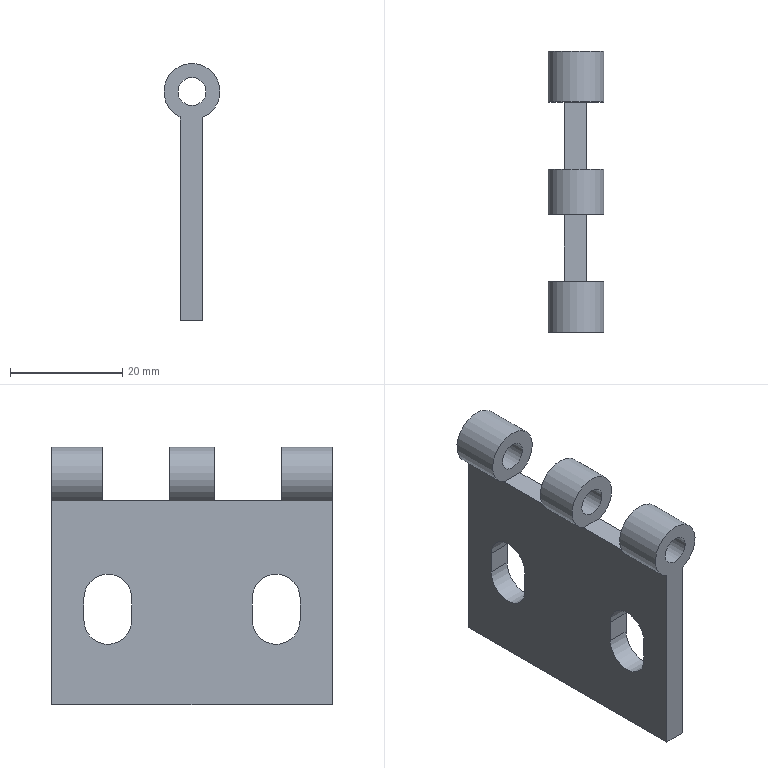Part | NX | features solid 2 | 1 solid | 24 faces | box 10 x 50 x 45.793 mm | volume 8023 mm3 | plane 14 | cylinder 10 | commonest cylinder face diameters 8.5 x4 5 x3 10 x3
STEP:
#1=CARTESIAN_POINT('',(-1603.983,496.,11.257));
#2=VERTEX_POINT('',#1);
#3=CARTESIAN_POINT('',(-1603.983,505.,11.257));
#4=VERTEX_POINT('',#3);
#5=CARTESIAN_POINT('',(-1603.983,485.,11.257));
#6=DIRECTION('',(0.,1.,0.));
#7=VECTOR('',#6,1000.);
#8=LINE('',#5,#7);
#9=EDGE_CURVE('',#2,#4,#8,.T.);
#10=ORIENTED_EDGE('',*,*,#9,.T.);
#11=CARTESIAN_POINT('',(-1604.,505.,11.257));
#12=VERTEX_POINT('',#11);
#13=CARTESIAN_POINT('',(-1604.,505.,11.257));
#14=DIRECTION('',(1.,0.,0.));
#15=VECTOR('',#14,1000.);
#16=LINE('',#13,#15);
#17=EDGE_CURVE('',#12,#4,#16,.T.);
#18=ORIENTED_EDGE('',*,*,#17,.F.);
#19=CARTESIAN_POINT('',(-1604.,455.,11.257));
#20=VERTEX_POINT('',#19);
#21=CARTESIAN_POINT('',(-1604.,505.,11.257));
#22=DIRECTION('',(0.,1.,0.));
#23=VECTOR('',#22,1000.);
#24=LINE('',#21,#23);
#25=EDGE_CURVE('',#12,#20,#24,.F.);
#26=ORIENTED_EDGE('',*,*,#25,.T.);
#27=CARTESIAN_POINT('',(-1603.983,455.,11.257));
#28=VERTEX_POINT('',#27);
#29=CARTESIAN_POINT('',(-1604.,455.,11.257));
#30=DIRECTION('',(1.,0.,0.));
#31=VECTOR('',#30,1000.);
#32=LINE('',#29,#31);
#33=EDGE_CURVE('',#20,#28,#32,.T.);
#34=ORIENTED_EDGE('',*,*,#33,.T.);
#35=CARTESIAN_POINT('',(-1603.983,464.,11.257));
#36=VERTEX_POINT('',#35);
#37=CARTESIAN_POINT('',(-1603.983,445.,11.257));
#38=DIRECTION('',(0.,1.,0.));
#39=VECTOR('',#38,1000.);
#40=LINE('',#37,#39);
#41=EDGE_CURVE('',#28,#36,#40,.T.);
#42=ORIENTED_EDGE('',*,*,#41,.T.);
#43=CARTESIAN_POINT('',(-1600.,464.,11.257));
#44=VERTEX_POINT('',#43);
#45=CARTESIAN_POINT('',(-1604.,464.,11.257));
#46=DIRECTION('',(1.,0.,0.));
#47=VECTOR('',#46,1000.);
#48=LINE('',#45,#47);
#49=EDGE_CURVE('',#36,#44,#48,.T.);
#50=ORIENTED_EDGE('',*,*,#49,.T.);
#51=CARTESIAN_POINT('',(-1600.,476.,11.257));
#52=VERTEX_POINT('',#51);
#53=CARTESIAN_POINT('',(-1600.,505.,11.257));
#54=DIRECTION('',(0.,1.,0.));
#55=VECTOR('',#54,1000.);
#56=LINE('',#53,#55);
#57=EDGE_CURVE('',#52,#44,#56,.F.);
#58=ORIENTED_EDGE('',*,*,#57,.F.);
#59=CARTESIAN_POINT('',(-1603.983,476.,11.257));
#60=VERTEX_POINT('',#59);
#61=CARTESIAN_POINT('',(-1604.,476.,11.257));
#62=DIRECTION('',(1.,0.,0.));
#63=VECTOR('',#62,1000.);
#64=LINE('',#61,#63);
#65=EDGE_CURVE('',#60,#52,#64,.T.);
#66=ORIENTED_EDGE('',*,*,#65,.F.);
#67=CARTESIAN_POINT('',(-1603.983,484.,11.257));
#68=VERTEX_POINT('',#67);
#69=CARTESIAN_POINT('',(-1603.983,465.,11.257));
#70=DIRECTION('',(0.,1.,0.));
#71=VECTOR('',#70,1000.);
#72=LINE('',#69,#71);
#73=EDGE_CURVE('',#60,#68,#72,.T.);
#74=ORIENTED_EDGE('',*,*,#73,.T.);
#75=CARTESIAN_POINT('',(-1600.,484.,11.257));
#76=VERTEX_POINT('',#75);
#77=CARTESIAN_POINT('',(-1604.,484.,11.257));
#78=DIRECTION('',(1.,0.,0.));
#79=VECTOR('',#78,1000.);
#80=LINE('',#77,#79);
#81=EDGE_CURVE('',#68,#76,#80,.T.);
#82=ORIENTED_EDGE('',*,*,#81,.T.);
#83=CARTESIAN_POINT('',(-1600.,496.,11.257));
#84=VERTEX_POINT('',#83);
#85=CARTESIAN_POINT('',(-1600.,505.,11.257));
#86=DIRECTION('',(0.,1.,0.));
#87=VECTOR('',#86,1000.);
#88=LINE('',#85,#87);
#89=EDGE_CURVE('',#84,#76,#88,.F.);
#90=ORIENTED_EDGE('',*,*,#89,.F.);
#91=CARTESIAN_POINT('',(-1604.,496.,11.257));
#92=DIRECTION('',(1.,0.,0.));
#93=VECTOR('',#92,1000.);
#94=LINE('',#91,#93);
#95=EDGE_CURVE('',#2,#84,#94,.T.);
#96=ORIENTED_EDGE('',*,*,#95,.F.);
#97=EDGE_LOOP('',(#10,#18,#26,#34,#42,#50,#58,#66,#74,#82,#90,#96));
#98=FACE_BOUND('',#97,.T.);
#99=CARTESIAN_POINT('',(-1604.,505.,11.257));
#100=DIRECTION('',(0.,0.,-1.));
#101=DIRECTION('',(0.,-1.,0.));
#102=AXIS2_PLACEMENT_3D('',#99,#100,#101);
#103=PLANE('',#102);
#104=ADVANCED_FACE('',(#98),#103,.F.);
#105=CARTESIAN_POINT('',(-1600.,490.75,-10.));
#106=VERTEX_POINT('',#105);
#107=CARTESIAN_POINT('',(-1600.,490.75,-6.));
#108=VERTEX_POINT('',#107);
#109=CARTESIAN_POINT('',(-1600.,490.75,-10.));
#110=DIRECTION('',(0.,0.,1.));
#111=VECTOR('',#110,1000.);
#112=LINE('',#109,#111);
#113=EDGE_CURVE('',#106,#108,#112,.T.);
#114=ORIENTED_EDGE('',*,*,#113,.T.);
#115=CARTESIAN_POINT('',(-1600.,499.25,-6.));
#116=VERTEX_POINT('',#115);
#117=CARTESIAN_POINT('',(-1600.,495.,-6.));
#118=DIRECTION('',(1.,0.,0.));
#119=DIRECTION('',(0.,0.,-1.));
#120=AXIS2_PLACEMENT_3D('',#117,#118,#119);
#121=CIRCLE('',#120,4.25);
#122=EDGE_CURVE('',#116,#108,#121,.T.);
#123=ORIENTED_EDGE('',*,*,#122,.F.);
#124=CARTESIAN_POINT('',(-1600.,499.25,-10.));
#125=VERTEX_POINT('',#124);
#126=CARTESIAN_POINT('',(-1600.,499.25,-10.));
#127=DIRECTION('',(0.,0.,1.));
#128=VECTOR('',#127,1000.);
#129=LINE('',#126,#128);
#130=EDGE_CURVE('',#125,#116,#129,.T.);
#131=ORIENTED_EDGE('',*,*,#130,.F.);
#132=CARTESIAN_POINT('',(-1600.,495.,-10.));
#133=DIRECTION('',(1.,0.,0.));
#134=DIRECTION('',(0.,0.,-1.));
#135=AXIS2_PLACEMENT_3D('',#132,#133,#134);
#136=CIRCLE('',#135,4.25);
#137=EDGE_CURVE('',#106,#125,#136,.T.);
#138=ORIENTED_EDGE('',*,*,#137,.F.);
#139=EDGE_LOOP('',(#114,#123,#131,#138));
#140=FACE_BOUND('',#139,.T.);
#141=CARTESIAN_POINT('',(-1600.,460.75,-10.));
#142=VERTEX_POINT('',#141);
#143=CARTESIAN_POINT('',(-1600.,460.75,-6.));
#144=VERTEX_POINT('',#143);
#145=CARTESIAN_POINT('',(-1600.,460.75,-10.));
#146=DIRECTION('',(0.,0.,1.));
#147=VECTOR('',#146,1000.);
#148=LINE('',#145,#147);
#149=EDGE_CURVE('',#142,#144,#148,.T.);
#150=ORIENTED_EDGE('',*,*,#149,.T.);
#151=CARTESIAN_POINT('',(-1600.,469.25,-6.));
#152=VERTEX_POINT('',#151);
#153=CARTESIAN_POINT('',(-1600.,465.,-6.));
#154=DIRECTION('',(1.,0.,0.));
#155=DIRECTION('',(0.,0.,-1.));
#156=AXIS2_PLACEMENT_3D('',#153,#154,#155);
#157=CIRCLE('',#156,4.25);
#158=EDGE_CURVE('',#152,#144,#157,.T.);
#159=ORIENTED_EDGE('',*,*,#158,.F.);
#160=CARTESIAN_POINT('',(-1600.,469.25,-10.));
#161=VERTEX_POINT('',#160);
#162=CARTESIAN_POINT('',(-1600.,469.25,-10.));
#163=DIRECTION('',(0.,0.,1.));
#164=VECTOR('',#163,1000.);
#165=LINE('',#162,#164);
#166=EDGE_CURVE('',#161,#152,#165,.T.);
#167=ORIENTED_EDGE('',*,*,#166,.F.);
#168=CARTESIAN_POINT('',(-1600.,465.,-10.));
#169=DIRECTION('',(1.,0.,0.));
#170=DIRECTION('',(0.,0.,-1.));
#171=AXIS2_PLACEMENT_3D('',#168,#169,#170);
#172=CIRCLE('',#171,4.25);
#173=EDGE_CURVE('',#142,#161,#172,.T.);
#174=ORIENTED_EDGE('',*,*,#173,.F.);
#175=EDGE_LOOP('',(#150,#159,#167,#174));
#176=FACE_BOUND('',#175,.T.);
#177=CARTESIAN_POINT('',(-1600.,496.,11.159));
#178=VERTEX_POINT('',#177);
#179=CARTESIAN_POINT('',(-1600.,496.,-39.243));
#180=DIRECTION('',(0.,0.,-1.));
#181=VECTOR('',#180,1000.);
#182=LINE('',#179,#181);
#183=EDGE_CURVE('',#178,#84,#182,.F.);
#184=ORIENTED_EDGE('',*,*,#183,.T.);
#185=ORIENTED_EDGE('',*,*,#89,.T.);
#186=CARTESIAN_POINT('',(-1600.,484.,11.159));
#187=VERTEX_POINT('',#186);
#188=CARTESIAN_POINT('',(-1600.,484.,-39.243));
#189=DIRECTION('',(0.,0.,-1.));
#190=VECTOR('',#189,1000.);
#191=LINE('',#188,#190);
#192=EDGE_CURVE('',#187,#76,#191,.F.);
#193=ORIENTED_EDGE('',*,*,#192,.F.);
#194=CARTESIAN_POINT('',(-1600.,476.,11.159));
#195=VERTEX_POINT('',#194);
#196=CARTESIAN_POINT('',(-1600.,465.,11.159));
#197=DIRECTION('',(0.,1.,0.));
#198=VECTOR('',#197,1000.);
#199=LINE('',#196,#198);
#200=EDGE_CURVE('',#195,#187,#199,.T.);
#201=ORIENTED_EDGE('',*,*,#200,.F.);
#202=CARTESIAN_POINT('',(-1600.,476.,-39.243));
#203=DIRECTION('',(0.,0.,-1.));
#204=VECTOR('',#203,1000.);
#205=LINE('',#202,#204);
#206=EDGE_CURVE('',#195,#52,#205,.F.);
#207=ORIENTED_EDGE('',*,*,#206,.T.);
#208=ORIENTED_EDGE('',*,*,#57,.T.);
#209=CARTESIAN_POINT('',(-1600.,464.,11.159));
#210=VERTEX_POINT('',#209);
#211=CARTESIAN_POINT('',(-1600.,464.,-39.243));
#212=DIRECTION('',(0.,0.,-1.));
#213=VECTOR('',#212,1000.);
#214=LINE('',#211,#213);
#215=EDGE_CURVE('',#210,#44,#214,.F.);
#216=ORIENTED_EDGE('',*,*,#215,.F.);
#217=CARTESIAN_POINT('',(-1600.,455.,11.159));
#218=VERTEX_POINT('',#217);
#219=CARTESIAN_POINT('',(-1600.,445.,11.159));
#220=DIRECTION('',(0.,1.,0.));
#221=VECTOR('',#220,1000.);
#222=LINE('',#219,#221);
#223=EDGE_CURVE('',#218,#210,#222,.T.);
#224=ORIENTED_EDGE('',*,*,#223,.F.);
#225=CARTESIAN_POINT('',(-1600.,455.,-25.));
#226=VERTEX_POINT('',#225);
#227=CARTESIAN_POINT('',(-1600.,455.,-39.243));
#228=DIRECTION('',(0.,0.,-1.));
#229=VECTOR('',#228,1000.);
#230=LINE('',#227,#229);
#231=EDGE_CURVE('',#226,#218,#230,.F.);
#232=ORIENTED_EDGE('',*,*,#231,.F.);
#233=CARTESIAN_POINT('',(-1600.,505.,-25.));
#234=VERTEX_POINT('',#233);
#235=CARTESIAN_POINT('',(-1600.,505.,-25.));
#236=DIRECTION('',(0.,1.,0.));
#237=VECTOR('',#236,1000.);
#238=LINE('',#235,#237);
#239=EDGE_CURVE('',#234,#226,#238,.F.);
#240=ORIENTED_EDGE('',*,*,#239,.F.);
#241=CARTESIAN_POINT('',(-1600.,505.,11.159));
#242=VERTEX_POINT('',#241);
#243=CARTESIAN_POINT('',(-1600.,505.,-39.243));
#244=DIRECTION('',(0.,0.,-1.));
#245=VECTOR('',#244,1000.);
#246=LINE('',#243,#245);
#247=EDGE_CURVE('',#234,#242,#246,.F.);
#248=ORIENTED_EDGE('',*,*,#247,.T.);
#249=CARTESIAN_POINT('',(-1600.,485.,11.159));
#250=DIRECTION('',(0.,1.,0.));
#251=VECTOR('',#250,1000.);
#252=LINE('',#249,#251);
#253=EDGE_CURVE('',#178,#242,#252,.T.);
#254=ORIENTED_EDGE('',*,*,#253,.F.);
#255=EDGE_LOOP('',(#184,#185,#193,#201,#207,#208,#216,#224,#232,#240,#248,#254));
#256=FACE_BOUND('',#255,.T.);
#257=CARTESIAN_POINT('',(-1600.,505.,-39.243));
#258=DIRECTION('',(-1.,0.,0.));
#259=DIRECTION('',(0.,-1.,0.));
#260=AXIS2_PLACEMENT_3D('',#257,#258,#259);
#261=PLANE('',#260);
#262=ADVANCED_FACE('',(#140,#176,#256),#261,.F.);
#263=ORIENTED_EDGE('',*,*,#239,.T.);
#264=CARTESIAN_POINT('',(-1604.,455.,-25.));
#265=VERTEX_POINT('',#264);
#266=CARTESIAN_POINT('',(-1604.,455.,-25.));
#267=CARTESIAN_POINT('',(-1602.667,455.,-25.));
#268=CARTESIAN_POINT('',(-1601.333,455.,-25.));
#269=CARTESIAN_POINT('',(-1600.,455.,-25.));
#270=B_SPLINE_CURVE_WITH_KNOTS('',3,(#266,#267,#268,#269),.UNSPECIFIED.,.F.,.F.,(4,4),(0.,1.),.UNSPECIFIED.);
#271=EDGE_CURVE('',#265,#226,#270,.T.);
#272=ORIENTED_EDGE('',*,*,#271,.F.);
#273=CARTESIAN_POINT('',(-1604.,505.,-25.));
#274=VERTEX_POINT('',#273);
#275=CARTESIAN_POINT('',(-1604.,505.,-25.));
#276=DIRECTION('',(0.,1.,0.));
#277=VECTOR('',#276,1000.);
#278=LINE('',#275,#277);
#279=EDGE_CURVE('',#274,#265,#278,.F.);
#280=ORIENTED_EDGE('',*,*,#279,.F.);
#281=CARTESIAN_POINT('',(-1600.,505.,-25.));
#282=CARTESIAN_POINT('',(-1601.333,505.,-25.));
#283=CARTESIAN_POINT('',(-1602.667,505.,-25.));
#284=CARTESIAN_POINT('',(-1604.,505.,-25.));
#285=B_SPLINE_CURVE_WITH_KNOTS('',3,(#281,#282,#283,#284),.UNSPECIFIED.,.F.,.F.,(4,4),(0.,1.),.UNSPECIFIED.);
#286=EDGE_CURVE('',#274,#234,#285,.F.);
#287=ORIENTED_EDGE('',*,*,#286,.T.);
#288=EDGE_LOOP('',(#263,#272,#280,#287));
#289=FACE_BOUND('',#288,.T.);
#290=CARTESIAN_POINT('',(-1604.,505.,-25.));
#291=DIRECTION('',(0.,0.,-1.));
#292=DIRECTION('',(0.,-1.,0.));
#293=AXIS2_PLACEMENT_3D('',#290,#291,#292);
#294=PLANE('',#293);
#295=ADVANCED_FACE('',(#289),#294,.T.);
#296=CARTESIAN_POINT('',(-1601.879,505.,15.793));
#297=DIRECTION('',(0.,1.,0.));
#298=DIRECTION('',(0.,0.,1.));
#299=AXIS2_PLACEMENT_3D('',#296,#297,#298);
#300=CIRCLE('',#299,5.);
#301=EDGE_CURVE('',#4,#242,#300,.T.);
#302=ORIENTED_EDGE('',*,*,#301,.T.);
#303=ORIENTED_EDGE('',*,*,#247,.F.);
#304=ORIENTED_EDGE('',*,*,#286,.F.);
#305=CARTESIAN_POINT('',(-1604.,505.,-39.243));
#306=DIRECTION('',(0.,0.,-1.));
#307=VECTOR('',#306,1000.);
#308=LINE('',#305,#307);
#309=EDGE_CURVE('',#274,#12,#308,.F.);
#310=ORIENTED_EDGE('',*,*,#309,.T.);
#311=ORIENTED_EDGE('',*,*,#17,.T.);
#312=EDGE_LOOP('',(#302,#303,#304,#310,#311));
#313=FACE_BOUND('',#312,.T.);
#314=CARTESIAN_POINT('',(-1601.879,505.,18.293));
#315=VERTEX_POINT('',#314);
#316=CARTESIAN_POINT('',(-1601.879,505.,15.793));
#317=DIRECTION('',(0.,1.,0.));
#318=DIRECTION('',(0.,0.,1.));
#319=AXIS2_PLACEMENT_3D('',#316,#317,#318);
#320=CIRCLE('',#319,2.5);
#321=EDGE_CURVE('',#315,#315,#320,.T.);
#322=ORIENTED_EDGE('',*,*,#321,.F.);
#323=EDGE_LOOP('',(#322));
#324=FACE_BOUND('',#323,.T.);
#325=CARTESIAN_POINT('',(-1604.,505.,-39.243));
#326=DIRECTION('',(0.,-1.,0.));
#327=DIRECTION('',(0.,0.,1.));
#328=AXIS2_PLACEMENT_3D('',#325,#326,#327);
#329=PLANE('',#328);
#330=ADVANCED_FACE('',(#313,#324),#329,.F.);
#331=CARTESIAN_POINT('',(-1601.879,455.,15.793));
#332=DIRECTION('',(0.,1.,0.));
#333=DIRECTION('',(0.,0.,1.));
#334=AXIS2_PLACEMENT_3D('',#331,#332,#333);
#335=CIRCLE('',#334,5.);
#336=EDGE_CURVE('',#28,#218,#335,.T.);
#337=ORIENTED_EDGE('',*,*,#336,.F.);
#338=ORIENTED_EDGE('',*,*,#33,.F.);
#339=CARTESIAN_POINT('',(-1604.,455.,-39.243));
#340=DIRECTION('',(0.,0.,-1.));
#341=VECTOR('',#340,1000.);
#342=LINE('',#339,#341);
#343=EDGE_CURVE('',#265,#20,#342,.F.);
#344=ORIENTED_EDGE('',*,*,#343,.F.);
#345=ORIENTED_EDGE('',*,*,#271,.T.);
#346=ORIENTED_EDGE('',*,*,#231,.T.);
#347=EDGE_LOOP('',(#337,#338,#344,#345,#346));
#348=FACE_BOUND('',#347,.T.);
#349=CARTESIAN_POINT('',(-1601.879,455.,18.293));
#350=VERTEX_POINT('',#349);
#351=CARTESIAN_POINT('',(-1601.879,455.,15.793));
#352=DIRECTION('',(0.,1.,0.));
#353=DIRECTION('',(0.,0.,1.));
#354=AXIS2_PLACEMENT_3D('',#351,#352,#353);
#355=CIRCLE('',#354,2.5);
#356=EDGE_CURVE('',#350,#350,#355,.T.);
#357=ORIENTED_EDGE('',*,*,#356,.T.);
#358=EDGE_LOOP('',(#357));
#359=FACE_BOUND('',#358,.T.);
#360=CARTESIAN_POINT('',(-1604.,455.,-39.243));
#361=DIRECTION('',(0.,-1.,0.));
#362=DIRECTION('',(0.,0.,1.));
#363=AXIS2_PLACEMENT_3D('',#360,#361,#362);
#364=PLANE('',#363);
#365=ADVANCED_FACE('',(#348,#359),#364,.T.);
#366=CARTESIAN_POINT('',(-1604.,490.75,-10.));
#367=VERTEX_POINT('',#366);
#368=CARTESIAN_POINT('',(-1604.,499.25,-10.));
#369=VERTEX_POINT('',#368);
#370=CARTESIAN_POINT('',(-1604.,495.,-10.));
#371=DIRECTION('',(1.,0.,0.));
#372=DIRECTION('',(0.,0.,-1.));
#373=AXIS2_PLACEMENT_3D('',#370,#371,#372);
#374=CIRCLE('',#373,4.25);
#375=EDGE_CURVE('',#367,#369,#374,.T.);
#376=ORIENTED_EDGE('',*,*,#375,.T.);
#377=CARTESIAN_POINT('',(-1604.,499.25,-6.));
#378=VERTEX_POINT('',#377);
#379=CARTESIAN_POINT('',(-1604.,499.25,-8.));
#380=DIRECTION('',(0.,0.,1.));
#381=VECTOR('',#380,1000.);
#382=LINE('',#379,#381);
#383=EDGE_CURVE('',#369,#378,#382,.T.);
#384=ORIENTED_EDGE('',*,*,#383,.T.);
#385=CARTESIAN_POINT('',(-1604.,490.75,-6.));
#386=VERTEX_POINT('',#385);
#387=CARTESIAN_POINT('',(-1604.,495.,-6.));
#388=DIRECTION('',(1.,0.,0.));
#389=DIRECTION('',(0.,0.,-1.));
#390=AXIS2_PLACEMENT_3D('',#387,#388,#389);
#391=CIRCLE('',#390,4.25);
#392=EDGE_CURVE('',#378,#386,#391,.T.);
#393=ORIENTED_EDGE('',*,*,#392,.T.);
#394=CARTESIAN_POINT('',(-1604.,490.75,-8.));
#395=DIRECTION('',(0.,0.,1.));
#396=VECTOR('',#395,1000.);
#397=LINE('',#394,#396);
#398=EDGE_CURVE('',#367,#386,#397,.T.);
#399=ORIENTED_EDGE('',*,*,#398,.F.);
#400=EDGE_LOOP('',(#376,#384,#393,#399));
#401=FACE_BOUND('',#400,.T.);
#402=CARTESIAN_POINT('',(-1604.,460.75,-10.));
#403=VERTEX_POINT('',#402);
#404=CARTESIAN_POINT('',(-1604.,469.25,-10.));
#405=VERTEX_POINT('',#404);
#406=CARTESIAN_POINT('',(-1604.,465.,-10.));
#407=DIRECTION('',(1.,0.,0.));
#408=DIRECTION('',(0.,0.,-1.));
#409=AXIS2_PLACEMENT_3D('',#406,#407,#408);
#410=CIRCLE('',#409,4.25);
#411=EDGE_CURVE('',#403,#405,#410,.T.);
#412=ORIENTED_EDGE('',*,*,#411,.T.);
#413=CARTESIAN_POINT('',(-1604.,469.25,-6.));
#414=VERTEX_POINT('',#413);
#415=CARTESIAN_POINT('',(-1604.,469.25,-8.));
#416=DIRECTION('',(0.,0.,1.));
#417=VECTOR('',#416,1000.);
#418=LINE('',#415,#417);
#419=EDGE_CURVE('',#405,#414,#418,.T.);
#420=ORIENTED_EDGE('',*,*,#419,.T.);
#421=CARTESIAN_POINT('',(-1604.,460.75,-6.));
#422=VERTEX_POINT('',#421);
#423=CARTESIAN_POINT('',(-1604.,465.,-6.));
#424=DIRECTION('',(1.,0.,0.));
#425=DIRECTION('',(0.,0.,-1.));
#426=AXIS2_PLACEMENT_3D('',#423,#424,#425);
#427=CIRCLE('',#426,4.25);
#428=EDGE_CURVE('',#414,#422,#427,.T.);
#429=ORIENTED_EDGE('',*,*,#428,.T.);
#430=CARTESIAN_POINT('',(-1604.,460.75,-8.));
#431=DIRECTION('',(0.,0.,1.));
#432=VECTOR('',#431,1000.);
#433=LINE('',#430,#432);
#434=EDGE_CURVE('',#403,#422,#433,.T.);
#435=ORIENTED_EDGE('',*,*,#434,.F.);
#436=EDGE_LOOP('',(#412,#420,#429,#435));
#437=FACE_BOUND('',#436,.T.);
#438=ORIENTED_EDGE('',*,*,#279,.T.);
#439=ORIENTED_EDGE('',*,*,#343,.T.);
#440=ORIENTED_EDGE('',*,*,#25,.F.);
#441=ORIENTED_EDGE('',*,*,#309,.F.);
#442=EDGE_LOOP('',(#438,#439,#440,#441));
#443=FACE_BOUND('',#442,.T.);
#444=CARTESIAN_POINT('',(-1604.,505.,-39.243));
#445=DIRECTION('',(-1.,0.,0.));
#446=DIRECTION('',(0.,-1.,0.));
#447=AXIS2_PLACEMENT_3D('',#444,#445,#446);
#448=PLANE('',#447);
#449=ADVANCED_FACE('',(#401,#437,#443),#448,.T.);
#450=ORIENTED_EDGE('',*,*,#336,.T.);
#451=ORIENTED_EDGE('',*,*,#223,.T.);
#452=CARTESIAN_POINT('',(-1601.879,464.,15.793));
#453=DIRECTION('',(0.,1.,0.));
#454=DIRECTION('',(0.,0.,1.));
#455=AXIS2_PLACEMENT_3D('',#452,#453,#454);
#456=CIRCLE('',#455,5.);
#457=EDGE_CURVE('',#36,#210,#456,.T.);
#458=ORIENTED_EDGE('',*,*,#457,.F.);
#459=ORIENTED_EDGE('',*,*,#41,.F.);
#460=EDGE_LOOP('',(#450,#451,#458,#459));
#461=FACE_BOUND('',#460,.T.);
#462=CARTESIAN_POINT('',(-1601.879,445.,15.793));
#463=DIRECTION('',(0.,1.,0.));
#464=DIRECTION('',(0.,0.,-1.));
#465=AXIS2_PLACEMENT_3D('',#462,#463,#464);
#466=CYLINDRICAL_SURFACE('',#465,5.);
#467=ADVANCED_FACE('',(#461),#466,.T.);
#468=CARTESIAN_POINT('',(-1601.879,464.,18.293));
#469=VERTEX_POINT('',#468);
#470=CARTESIAN_POINT('',(-1601.879,464.,15.793));
#471=DIRECTION('',(0.,1.,0.));
#472=DIRECTION('',(0.,0.,1.));
#473=AXIS2_PLACEMENT_3D('',#470,#471,#472);
#474=CIRCLE('',#473,2.5);
#475=EDGE_CURVE('',#469,#469,#474,.T.);
#476=ORIENTED_EDGE('',*,*,#475,.F.);
#477=EDGE_LOOP('',(#476));
#478=FACE_BOUND('',#477,.T.);
#479=ORIENTED_EDGE('',*,*,#457,.T.);
#480=ORIENTED_EDGE('',*,*,#215,.T.);
#481=ORIENTED_EDGE('',*,*,#49,.F.);
#482=EDGE_LOOP('',(#479,#480,#481));
#483=FACE_BOUND('',#482,.T.);
#484=CARTESIAN_POINT('',(-1601.879,464.,15.793));
#485=DIRECTION('',(0.,-1.,0.));
#486=DIRECTION('',(0.,0.,1.));
#487=AXIS2_PLACEMENT_3D('',#484,#485,#486);
#488=PLANE('',#487);
#489=ADVANCED_FACE('',(#478,#483),#488,.F.);
#490=ORIENTED_EDGE('',*,*,#356,.F.);
#491=EDGE_LOOP('',(#490));
#492=FACE_BOUND('',#491,.T.);
#493=ORIENTED_EDGE('',*,*,#475,.T.);
#494=EDGE_LOOP('',(#493));
#495=FACE_BOUND('',#494,.T.);
#496=CARTESIAN_POINT('',(-1601.879,465.,15.793));
#497=DIRECTION('',(0.,-1.,0.));
#498=DIRECTION('',(0.,0.,1.));
#499=AXIS2_PLACEMENT_3D('',#496,#497,#498);
#500=CYLINDRICAL_SURFACE('',#499,2.5);
#501=ADVANCED_FACE('',(#492,#495),#500,.F.);
#502=CARTESIAN_POINT('',(-1601.879,476.,15.793));
#503=DIRECTION('',(0.,1.,0.));
#504=DIRECTION('',(0.,0.,1.));
#505=AXIS2_PLACEMENT_3D('',#502,#503,#504);
#506=CIRCLE('',#505,5.);
#507=EDGE_CURVE('',#60,#195,#506,.T.);
#508=ORIENTED_EDGE('',*,*,#507,.T.);
#509=ORIENTED_EDGE('',*,*,#200,.T.);
#510=CARTESIAN_POINT('',(-1601.879,484.,15.793));
#511=DIRECTION('',(0.,1.,0.));
#512=DIRECTION('',(0.,0.,1.));
#513=AXIS2_PLACEMENT_3D('',#510,#511,#512);
#514=CIRCLE('',#513,5.);
#515=EDGE_CURVE('',#68,#187,#514,.T.);
#516=ORIENTED_EDGE('',*,*,#515,.F.);
#517=ORIENTED_EDGE('',*,*,#73,.F.);
#518=EDGE_LOOP('',(#508,#509,#516,#517));
#519=FACE_BOUND('',#518,.T.);
#520=CARTESIAN_POINT('',(-1601.879,465.,15.793));
#521=DIRECTION('',(0.,1.,0.));
#522=DIRECTION('',(0.,0.,-1.));
#523=AXIS2_PLACEMENT_3D('',#520,#521,#522);
#524=CYLINDRICAL_SURFACE('',#523,5.);
#525=ADVANCED_FACE('',(#519),#524,.T.);
#526=CARTESIAN_POINT('',(-1601.879,476.,18.293));
#527=VERTEX_POINT('',#526);
#528=CARTESIAN_POINT('',(-1601.879,476.,15.793));
#529=DIRECTION('',(0.,1.,0.));
#530=DIRECTION('',(0.,0.,1.));
#531=AXIS2_PLACEMENT_3D('',#528,#529,#530);
#532=CIRCLE('',#531,2.5);
#533=EDGE_CURVE('',#527,#527,#532,.T.);
#534=ORIENTED_EDGE('',*,*,#533,.T.);
#535=EDGE_LOOP('',(#534));
#536=FACE_BOUND('',#535,.T.);
#537=ORIENTED_EDGE('',*,*,#65,.T.);
#538=ORIENTED_EDGE('',*,*,#206,.F.);
#539=ORIENTED_EDGE('',*,*,#507,.F.);
#540=EDGE_LOOP('',(#537,#538,#539));
#541=FACE_BOUND('',#540,.T.);
#542=CARTESIAN_POINT('',(-1601.879,476.,15.793));
#543=DIRECTION('',(0.,-1.,0.));
#544=DIRECTION('',(0.,0.,1.));
#545=AXIS2_PLACEMENT_3D('',#542,#543,#544);
#546=PLANE('',#545);
#547=ADVANCED_FACE('',(#536,#541),#546,.T.);
#548=CARTESIAN_POINT('',(-1601.879,484.,18.293));
#549=VERTEX_POINT('',#548);
#550=CARTESIAN_POINT('',(-1601.879,484.,15.793));
#551=DIRECTION('',(0.,1.,0.));
#552=DIRECTION('',(0.,0.,1.));
#553=AXIS2_PLACEMENT_3D('',#550,#551,#552);
#554=CIRCLE('',#553,2.5);
#555=EDGE_CURVE('',#549,#549,#554,.T.);
#556=ORIENTED_EDGE('',*,*,#555,.F.);
#557=EDGE_LOOP('',(#556));
#558=FACE_BOUND('',#557,.T.);
#559=ORIENTED_EDGE('',*,*,#515,.T.);
#560=ORIENTED_EDGE('',*,*,#192,.T.);
#561=ORIENTED_EDGE('',*,*,#81,.F.);
#562=EDGE_LOOP('',(#559,#560,#561));
#563=FACE_BOUND('',#562,.T.);
#564=CARTESIAN_POINT('',(-1601.879,484.,15.793));
#565=DIRECTION('',(0.,-1.,0.));
#566=DIRECTION('',(0.,0.,1.));
#567=AXIS2_PLACEMENT_3D('',#564,#565,#566);
#568=PLANE('',#567);
#569=ADVANCED_FACE('',(#558,#563),#568,.F.);
#570=ORIENTED_EDGE('',*,*,#533,.F.);
#571=EDGE_LOOP('',(#570));
#572=FACE_BOUND('',#571,.T.);
#573=ORIENTED_EDGE('',*,*,#555,.T.);
#574=EDGE_LOOP('',(#573));
#575=FACE_BOUND('',#574,.T.);
#576=CARTESIAN_POINT('',(-1601.879,485.,15.793));
#577=DIRECTION('',(0.,-1.,0.));
#578=DIRECTION('',(0.,0.,1.));
#579=AXIS2_PLACEMENT_3D('',#576,#577,#578);
#580=CYLINDRICAL_SURFACE('',#579,2.5);
#581=ADVANCED_FACE('',(#572,#575),#580,.F.);
#582=CARTESIAN_POINT('',(-1601.879,496.,18.293));
#583=VERTEX_POINT('',#582);
#584=CARTESIAN_POINT('',(-1601.879,496.,15.793));
#585=DIRECTION('',(0.,1.,0.));
#586=DIRECTION('',(0.,0.,1.));
#587=AXIS2_PLACEMENT_3D('',#584,#585,#586);
#588=CIRCLE('',#587,2.5);
#589=EDGE_CURVE('',#583,#583,#588,.T.);
#590=ORIENTED_EDGE('',*,*,#589,.T.);
#591=EDGE_LOOP('',(#590));
#592=FACE_BOUND('',#591,.T.);
#593=ORIENTED_EDGE('',*,*,#95,.T.);
#594=ORIENTED_EDGE('',*,*,#183,.F.);
#595=CARTESIAN_POINT('',(-1601.879,496.,15.793));
#596=DIRECTION('',(0.,1.,0.));
#597=DIRECTION('',(0.,0.,1.));
#598=AXIS2_PLACEMENT_3D('',#595,#596,#597);
#599=CIRCLE('',#598,5.);
#600=EDGE_CURVE('',#2,#178,#599,.T.);
#601=ORIENTED_EDGE('',*,*,#600,.F.);
#602=EDGE_LOOP('',(#593,#594,#601));
#603=FACE_BOUND('',#602,.T.);
#604=CARTESIAN_POINT('',(-1601.879,496.,15.793));
#605=DIRECTION('',(0.,-1.,0.));
#606=DIRECTION('',(0.,0.,1.));
#607=AXIS2_PLACEMENT_3D('',#604,#605,#606);
#608=PLANE('',#607);
#609=ADVANCED_FACE('',(#592,#603),#608,.T.);
#610=ORIENTED_EDGE('',*,*,#600,.T.);
#611=ORIENTED_EDGE('',*,*,#253,.T.);
#612=ORIENTED_EDGE('',*,*,#301,.F.);
#613=ORIENTED_EDGE('',*,*,#9,.F.);
#614=EDGE_LOOP('',(#610,#611,#612,#613));
#615=FACE_BOUND('',#614,.T.);
#616=CARTESIAN_POINT('',(-1601.879,485.,15.793));
#617=DIRECTION('',(0.,1.,0.));
#618=DIRECTION('',(0.,0.,-1.));
#619=AXIS2_PLACEMENT_3D('',#616,#617,#618);
#620=CYLINDRICAL_SURFACE('',#619,5.);
#621=ADVANCED_FACE('',(#615),#620,.T.);
#622=ORIENTED_EDGE('',*,*,#589,.F.);
#623=EDGE_LOOP('',(#622));
#624=FACE_BOUND('',#623,.T.);
#625=ORIENTED_EDGE('',*,*,#321,.T.);
#626=EDGE_LOOP('',(#625));
#627=FACE_BOUND('',#626,.T.);
#628=CARTESIAN_POINT('',(-1601.879,505.,15.793));
#629=DIRECTION('',(0.,-1.,0.));
#630=DIRECTION('',(0.,0.,1.));
#631=AXIS2_PLACEMENT_3D('',#628,#629,#630);
#632=CYLINDRICAL_SURFACE('',#631,2.5);
#633=ADVANCED_FACE('',(#624,#627),#632,.F.);
#634=ORIENTED_EDGE('',*,*,#434,.T.);
#635=CARTESIAN_POINT('',(-1604.,460.75,-6.));
#636=DIRECTION('',(-1.,0.,0.));
#637=VECTOR('',#636,1000.);
#638=LINE('',#635,#637);
#639=EDGE_CURVE('',#144,#422,#638,.T.);
#640=ORIENTED_EDGE('',*,*,#639,.F.);
#641=ORIENTED_EDGE('',*,*,#149,.F.);
#642=CARTESIAN_POINT('',(-1604.,460.75,-10.));
#643=DIRECTION('',(-1.,0.,0.));
#644=VECTOR('',#643,1000.);
#645=LINE('',#642,#644);
#646=EDGE_CURVE('',#142,#403,#645,.T.);
#647=ORIENTED_EDGE('',*,*,#646,.T.);
#648=EDGE_LOOP('',(#634,#640,#641,#647));
#649=FACE_BOUND('',#648,.T.);
#650=CARTESIAN_POINT('',(-1604.,460.75,-8.));
#651=DIRECTION('',(0.,-1.,0.));
#652=DIRECTION('',(0.,0.,1.));
#653=AXIS2_PLACEMENT_3D('',#650,#651,#652);
#654=PLANE('',#653);
#655=ADVANCED_FACE('',(#649),#654,.F.);
#656=ORIENTED_EDGE('',*,*,#411,.F.);
#657=ORIENTED_EDGE('',*,*,#646,.F.);
#658=ORIENTED_EDGE('',*,*,#173,.T.);
#659=CARTESIAN_POINT('',(-1604.,469.25,-10.));
#660=DIRECTION('',(-1.,0.,0.));
#661=VECTOR('',#660,1000.);
#662=LINE('',#659,#661);
#663=EDGE_CURVE('',#161,#405,#662,.T.);
#664=ORIENTED_EDGE('',*,*,#663,.T.);
#665=EDGE_LOOP('',(#656,#657,#658,#664));
#666=FACE_BOUND('',#665,.T.);
#667=CARTESIAN_POINT('',(-1604.,465.,-10.));
#668=DIRECTION('',(-1.,0.,0.));
#669=DIRECTION('',(0.,0.,-1.));
#670=AXIS2_PLACEMENT_3D('',#667,#668,#669);
#671=CYLINDRICAL_SURFACE('',#670,4.25);
#672=ADVANCED_FACE('',(#666),#671,.F.);
#673=ORIENTED_EDGE('',*,*,#419,.F.);
#674=ORIENTED_EDGE('',*,*,#663,.F.);
#675=ORIENTED_EDGE('',*,*,#166,.T.);
#676=CARTESIAN_POINT('',(-1604.,469.25,-6.));
#677=DIRECTION('',(-1.,0.,0.));
#678=VECTOR('',#677,1000.);
#679=LINE('',#676,#678);
#680=EDGE_CURVE('',#152,#414,#679,.T.);
#681=ORIENTED_EDGE('',*,*,#680,.T.);
#682=EDGE_LOOP('',(#673,#674,#675,#681));
#683=FACE_BOUND('',#682,.T.);
#684=CARTESIAN_POINT('',(-1604.,469.25,-8.));
#685=DIRECTION('',(0.,1.,0.));
#686=DIRECTION('',(0.,0.,-1.));
#687=AXIS2_PLACEMENT_3D('',#684,#685,#686);
#688=PLANE('',#687);
#689=ADVANCED_FACE('',(#683),#688,.F.);
#690=ORIENTED_EDGE('',*,*,#428,.F.);
#691=ORIENTED_EDGE('',*,*,#680,.F.);
#692=ORIENTED_EDGE('',*,*,#158,.T.);
#693=ORIENTED_EDGE('',*,*,#639,.T.);
#694=EDGE_LOOP('',(#690,#691,#692,#693));
#695=FACE_BOUND('',#694,.T.);
#696=CARTESIAN_POINT('',(-1604.,465.,-6.));
#697=DIRECTION('',(-1.,0.,0.));
#698=DIRECTION('',(0.,0.,-1.));
#699=AXIS2_PLACEMENT_3D('',#696,#697,#698);
#700=CYLINDRICAL_SURFACE('',#699,4.25);
#701=ADVANCED_FACE('',(#695),#700,.F.);
#702=ORIENTED_EDGE('',*,*,#398,.T.);
#703=CARTESIAN_POINT('',(-1604.,490.75,-6.));
#704=DIRECTION('',(-1.,0.,0.));
#705=VECTOR('',#704,1000.);
#706=LINE('',#703,#705);
#707=EDGE_CURVE('',#108,#386,#706,.T.);
#708=ORIENTED_EDGE('',*,*,#707,.F.);
#709=ORIENTED_EDGE('',*,*,#113,.F.);
#710=CARTESIAN_POINT('',(-1604.,490.75,-10.));
#711=DIRECTION('',(-1.,0.,0.));
#712=VECTOR('',#711,1000.);
#713=LINE('',#710,#712);
#714=EDGE_CURVE('',#106,#367,#713,.T.);
#715=ORIENTED_EDGE('',*,*,#714,.T.);
#716=EDGE_LOOP('',(#702,#708,#709,#715));
#717=FACE_BOUND('',#716,.T.);
#718=CARTESIAN_POINT('',(-1604.,490.75,-8.));
#719=DIRECTION('',(0.,-1.,0.));
#720=DIRECTION('',(0.,0.,1.));
#721=AXIS2_PLACEMENT_3D('',#718,#719,#720);
#722=PLANE('',#721);
#723=ADVANCED_FACE('',(#717),#722,.F.);
#724=ORIENTED_EDGE('',*,*,#375,.F.);
#725=ORIENTED_EDGE('',*,*,#714,.F.);
#726=ORIENTED_EDGE('',*,*,#137,.T.);
#727=CARTESIAN_POINT('',(-1604.,499.25,-10.));
#728=DIRECTION('',(-1.,0.,0.));
#729=VECTOR('',#728,1000.);
#730=LINE('',#727,#729);
#731=EDGE_CURVE('',#125,#369,#730,.T.);
#732=ORIENTED_EDGE('',*,*,#731,.T.);
#733=EDGE_LOOP('',(#724,#725,#726,#732));
#734=FACE_BOUND('',#733,.T.);
#735=CARTESIAN_POINT('',(-1604.,495.,-10.));
#736=DIRECTION('',(-1.,0.,0.));
#737=DIRECTION('',(0.,0.,-1.));
#738=AXIS2_PLACEMENT_3D('',#735,#736,#737);
#739=CYLINDRICAL_SURFACE('',#738,4.25);
#740=ADVANCED_FACE('',(#734),#739,.F.);
#741=ORIENTED_EDGE('',*,*,#383,.F.);
#742=ORIENTED_EDGE('',*,*,#731,.F.);
#743=ORIENTED_EDGE('',*,*,#130,.T.);
#744=CARTESIAN_POINT('',(-1604.,499.25,-6.));
#745=DIRECTION('',(-1.,0.,0.));
#746=VECTOR('',#745,1000.);
#747=LINE('',#744,#746);
#748=EDGE_CURVE('',#116,#378,#747,.T.);
#749=ORIENTED_EDGE('',*,*,#748,.T.);
#750=EDGE_LOOP('',(#741,#742,#743,#749));
#751=FACE_BOUND('',#750,.T.);
#752=CARTESIAN_POINT('',(-1604.,499.25,-8.));
#753=DIRECTION('',(0.,1.,0.));
#754=DIRECTION('',(0.,0.,-1.));
#755=AXIS2_PLACEMENT_3D('',#752,#753,#754);
#756=PLANE('',#755);
#757=ADVANCED_FACE('',(#751),#756,.F.);
#758=ORIENTED_EDGE('',*,*,#392,.F.);
#759=ORIENTED_EDGE('',*,*,#748,.F.);
#760=ORIENTED_EDGE('',*,*,#122,.T.);
#761=ORIENTED_EDGE('',*,*,#707,.T.);
#762=EDGE_LOOP('',(#758,#759,#760,#761));
#763=FACE_BOUND('',#762,.T.);
#764=CARTESIAN_POINT('',(-1604.,495.,-6.));
#765=DIRECTION('',(-1.,0.,0.));
#766=DIRECTION('',(0.,0.,-1.));
#767=AXIS2_PLACEMENT_3D('',#764,#765,#766);
#768=CYLINDRICAL_SURFACE('',#767,4.25);
#769=ADVANCED_FACE('',(#763),#768,.F.);
#770=CLOSED_SHELL('',(#104,#262,#295,#330,#365,#449,#467,#489,#501,#525,#547,#569,#581,#609,#621,#633,#655,#672,#689,#701,#723,#740,#757,#769));
#771=MANIFOLD_SOLID_BREP('',#770);
#772=(LENGTH_UNIT()NAMED_UNIT(*)SI_UNIT(.MILLI.,.METRE.));
#773=UNCERTAINTY_MEASURE_WITH_UNIT(LENGTH_MEASURE(0.0508),#772,'','');
#774=(NAMED_UNIT(*)PLANE_ANGLE_UNIT()SI_UNIT($,.RADIAN.));
#775=(NAMED_UNIT(*)SI_UNIT($,.STERADIAN.)SOLID_ANGLE_UNIT());
#776=(GEOMETRIC_REPRESENTATION_CONTEXT(3)GLOBAL_UNCERTAINTY_ASSIGNED_CONTEXT((#773))GLOBAL_UNIT_ASSIGNED_CONTEXT((#772,#774,#775))REPRESENTATION_CONTEXT('',''));
#777=ADVANCED_BREP_SHAPE_REPRESENTATION('',(#771),#776);